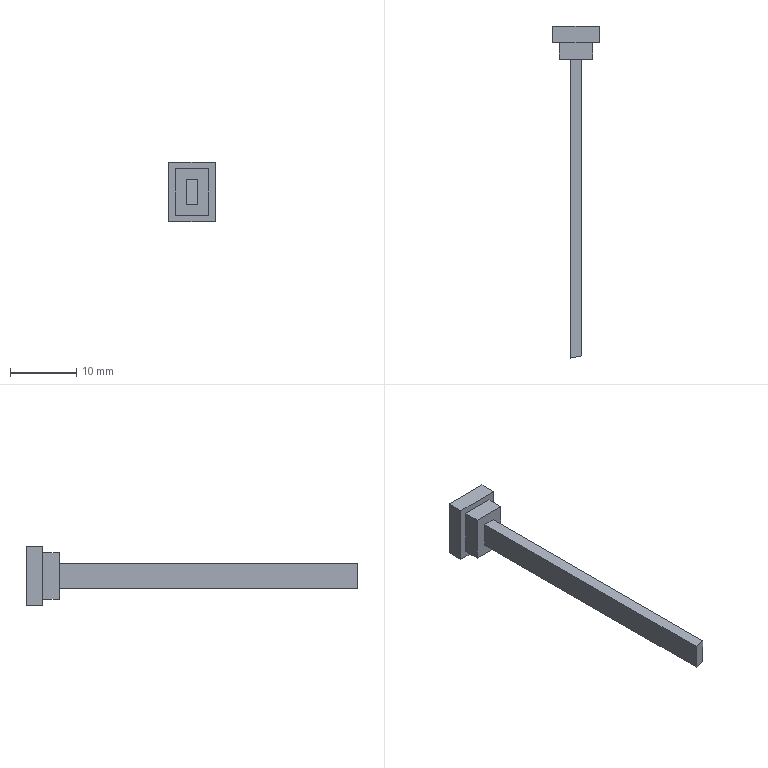Part | SolidWorks | features ICE 3, Extrusion 1 | 1 solid | 16 faces | box 7 x 50 x 9 mm | volume 546.722 mm3 | plane 16
STEP:
#1=CARTESIAN_POINT('',(-0.89,0.,-1.89));
#2=VERTEX_POINT('',#1);
#3=CARTESIAN_POINT('',(-0.89,0.,1.89));
#4=VERTEX_POINT('',#3);
#5=CARTESIAN_POINT('',(-0.89,0.,1.89));
#6=DIRECTION('',(0.,0.,1.));
#7=VECTOR('',#6,1000.);
#8=LINE('',#5,#7);
#9=EDGE_CURVE('',#2,#4,#8,.T.);
#10=ORIENTED_EDGE('',*,*,#9,.T.);
#11=CARTESIAN_POINT('',(-0.89,45.,1.89));
#12=VERTEX_POINT('',#11);
#13=CARTESIAN_POINT('',(-0.89,45.,1.89));
#14=DIRECTION('',(0.,-1.,0.));
#15=VECTOR('',#14,1000.);
#16=LINE('',#13,#15);
#17=EDGE_CURVE('',#12,#4,#16,.T.);
#18=ORIENTED_EDGE('',*,*,#17,.F.);
#19=CARTESIAN_POINT('',(-0.89,45.,-1.89));
#20=VERTEX_POINT('',#19);
#21=CARTESIAN_POINT('',(-0.89,45.,1.89));
#22=DIRECTION('',(0.,0.,1.));
#23=VECTOR('',#22,1000.);
#24=LINE('',#21,#23);
#25=EDGE_CURVE('',#20,#12,#24,.T.);
#26=ORIENTED_EDGE('',*,*,#25,.F.);
#27=CARTESIAN_POINT('',(-0.89,45.,-1.89));
#28=DIRECTION('',(0.,-1.,0.));
#29=VECTOR('',#28,1000.);
#30=LINE('',#27,#29);
#31=EDGE_CURVE('',#20,#2,#30,.T.);
#32=ORIENTED_EDGE('',*,*,#31,.T.);
#33=EDGE_LOOP('',(#10,#18,#26,#32));
#34=FACE_OUTER_BOUND('',#33,.T.);
#35=CARTESIAN_POINT('',(-0.89,45.,1.89));
#36=DIRECTION('',(1.,0.,0.));
#37=DIRECTION('',(0.,0.,-1.));
#38=AXIS2_PLACEMENT_3D('',#35,#36,#37);
#39=PLANE('',#38);
#40=ADVANCED_FACE('',(#34),#39,.F.);
#41=ORIENTED_EDGE('',*,*,#17,.T.);
#42=CARTESIAN_POINT('',(0.89,0.3139,1.89));
#43=VERTEX_POINT('',#42);
#44=CARTESIAN_POINT('',(0.89,0.3139,1.89));
#45=DIRECTION('',(-0.9848,-0.1736,0.));
#46=VECTOR('',#45,1000.);
#47=LINE('',#44,#46);
#48=EDGE_CURVE('',#43,#4,#47,.T.);
#49=ORIENTED_EDGE('',*,*,#48,.F.);
#50=CARTESIAN_POINT('',(0.89,45.,1.89));
#51=VERTEX_POINT('',#50);
#52=CARTESIAN_POINT('',(0.89,45.,1.89));
#53=DIRECTION('',(0.,-1.,0.));
#54=VECTOR('',#53,1000.);
#55=LINE('',#52,#54);
#56=EDGE_CURVE('',#51,#43,#55,.T.);
#57=ORIENTED_EDGE('',*,*,#56,.F.);
#58=CARTESIAN_POINT('',(0.89,45.,1.89));
#59=DIRECTION('',(1.,0.,0.));
#60=VECTOR('',#59,1000.);
#61=LINE('',#58,#60);
#62=EDGE_CURVE('',#12,#51,#61,.T.);
#63=ORIENTED_EDGE('',*,*,#62,.F.);
#64=EDGE_LOOP('',(#41,#49,#57,#63));
#65=FACE_OUTER_BOUND('',#64,.T.);
#66=CARTESIAN_POINT('',(0.89,45.,1.89));
#67=DIRECTION('',(0.,0.,-1.));
#68=DIRECTION('',(-1.,0.,0.));
#69=AXIS2_PLACEMENT_3D('',#66,#67,#68);
#70=PLANE('',#69);
#71=ADVANCED_FACE('',(#65),#70,.F.);
#72=ORIENTED_EDGE('',*,*,#56,.T.);
#73=CARTESIAN_POINT('',(0.89,0.3139,-1.89));
#74=VERTEX_POINT('',#73);
#75=CARTESIAN_POINT('',(0.89,0.3139,-1.89));
#76=DIRECTION('',(0.,0.,1.));
#77=VECTOR('',#76,1000.);
#78=LINE('',#75,#77);
#79=EDGE_CURVE('',#74,#43,#78,.T.);
#80=ORIENTED_EDGE('',*,*,#79,.F.);
#81=CARTESIAN_POINT('',(0.89,45.,-1.89));
#82=VERTEX_POINT('',#81);
#83=CARTESIAN_POINT('',(0.89,45.,-1.89));
#84=DIRECTION('',(0.,-1.,0.));
#85=VECTOR('',#84,1000.);
#86=LINE('',#83,#85);
#87=EDGE_CURVE('',#82,#74,#86,.T.);
#88=ORIENTED_EDGE('',*,*,#87,.F.);
#89=CARTESIAN_POINT('',(0.89,45.,-1.89));
#90=DIRECTION('',(0.,0.,-1.));
#91=VECTOR('',#90,1000.);
#92=LINE('',#89,#91);
#93=EDGE_CURVE('',#51,#82,#92,.T.);
#94=ORIENTED_EDGE('',*,*,#93,.F.);
#95=EDGE_LOOP('',(#72,#80,#88,#94));
#96=FACE_OUTER_BOUND('',#95,.T.);
#97=CARTESIAN_POINT('',(0.89,45.,-1.89));
#98=DIRECTION('',(-1.,0.,0.));
#99=DIRECTION('',(0.,0.,1.));
#100=AXIS2_PLACEMENT_3D('',#97,#98,#99);
#101=PLANE('',#100);
#102=ADVANCED_FACE('',(#96),#101,.F.);
#103=ORIENTED_EDGE('',*,*,#87,.T.);
#104=CARTESIAN_POINT('',(0.89,0.3139,-1.89));
#105=DIRECTION('',(-0.9848,-0.1736,0.));
#106=VECTOR('',#105,1000.);
#107=LINE('',#104,#106);
#108=EDGE_CURVE('',#74,#2,#107,.T.);
#109=ORIENTED_EDGE('',*,*,#108,.T.);
#110=ORIENTED_EDGE('',*,*,#31,.F.);
#111=CARTESIAN_POINT('',(-0.89,45.,-1.89));
#112=DIRECTION('',(-1.,0.,0.));
#113=VECTOR('',#112,1000.);
#114=LINE('',#111,#113);
#115=EDGE_CURVE('',#82,#20,#114,.T.);
#116=ORIENTED_EDGE('',*,*,#115,.F.);
#117=EDGE_LOOP('',(#103,#109,#110,#116));
#118=FACE_OUTER_BOUND('',#117,.T.);
#119=CARTESIAN_POINT('',(-0.89,45.,-1.89));
#120=DIRECTION('',(0.,0.,1.));
#121=DIRECTION('',(1.,0.,0.));
#122=AXIS2_PLACEMENT_3D('',#119,#120,#121);
#123=PLANE('',#122);
#124=ADVANCED_FACE('',(#118),#123,.F.);
#125=ORIENTED_EDGE('',*,*,#48,.T.);
#126=ORIENTED_EDGE('',*,*,#9,.F.);
#127=ORIENTED_EDGE('',*,*,#108,.F.);
#128=ORIENTED_EDGE('',*,*,#79,.T.);
#129=EDGE_LOOP('',(#125,#126,#127,#128));
#130=FACE_OUTER_BOUND('',#129,.T.);
#131=CARTESIAN_POINT('',(0.89,0.3139,-1.89));
#132=DIRECTION('',(-0.1736,0.9848,0.));
#133=DIRECTION('',(-0.9848,-0.1736,0.));
#134=AXIS2_PLACEMENT_3D('',#131,#132,#133);
#135=PLANE('',#134);
#136=ADVANCED_FACE('',(#130),#135,.F.);
#137=CARTESIAN_POINT('',(-2.5,45.,-3.5));
#138=VERTEX_POINT('',#137);
#139=CARTESIAN_POINT('',(-2.5,45.,3.5));
#140=VERTEX_POINT('',#139);
#141=CARTESIAN_POINT('',(-2.5,45.,-3.5));
#142=DIRECTION('',(0.,0.,1.));
#143=VECTOR('',#142,1000.);
#144=LINE('',#141,#143);
#145=EDGE_CURVE('',#138,#140,#144,.T.);
#146=ORIENTED_EDGE('',*,*,#145,.F.);
#147=CARTESIAN_POINT('',(2.5,45.,-3.5));
#148=VERTEX_POINT('',#147);
#149=CARTESIAN_POINT('',(-2.5,45.,-3.5));
#150=DIRECTION('',(-1.,0.,0.));
#151=VECTOR('',#150,1000.);
#152=LINE('',#149,#151);
#153=EDGE_CURVE('',#148,#138,#152,.T.);
#154=ORIENTED_EDGE('',*,*,#153,.F.);
#155=CARTESIAN_POINT('',(2.5,45.,3.5));
#156=VERTEX_POINT('',#155);
#157=CARTESIAN_POINT('',(2.5,45.,-3.5));
#158=DIRECTION('',(0.,0.,-1.));
#159=VECTOR('',#158,1000.);
#160=LINE('',#157,#159);
#161=EDGE_CURVE('',#156,#148,#160,.T.);
#162=ORIENTED_EDGE('',*,*,#161,.F.);
#163=CARTESIAN_POINT('',(-2.5,45.,3.5));
#164=DIRECTION('',(1.,0.,0.));
#165=VECTOR('',#164,1000.);
#166=LINE('',#163,#165);
#167=EDGE_CURVE('',#140,#156,#166,.T.);
#168=ORIENTED_EDGE('',*,*,#167,.F.);
#169=EDGE_LOOP('',(#146,#154,#162,#168));
#170=FACE_OUTER_BOUND('',#169,.T.);
#171=ORIENTED_EDGE('',*,*,#115,.T.);
#172=ORIENTED_EDGE('',*,*,#25,.T.);
#173=ORIENTED_EDGE('',*,*,#62,.T.);
#174=ORIENTED_EDGE('',*,*,#93,.T.);
#175=EDGE_LOOP('',(#171,#172,#173,#174));
#176=FACE_BOUND('',#175,.T.);
#177=CARTESIAN_POINT('',(0.,45.,0.));
#178=DIRECTION('',(0.,1.,0.));
#179=DIRECTION('',(0.,0.,1.));
#180=AXIS2_PLACEMENT_3D('',#177,#178,#179);
#181=PLANE('',#180);
#182=ADVANCED_FACE('',(#170,#176),#181,.F.);
#183=ORIENTED_EDGE('',*,*,#145,.T.);
#184=CARTESIAN_POINT('',(-2.5,47.5,3.5));
#185=VERTEX_POINT('',#184);
#186=CARTESIAN_POINT('',(-2.5,47.5,3.5));
#187=DIRECTION('',(0.,-1.,0.));
#188=VECTOR('',#187,1000.);
#189=LINE('',#186,#188);
#190=EDGE_CURVE('',#185,#140,#189,.T.);
#191=ORIENTED_EDGE('',*,*,#190,.F.);
#192=CARTESIAN_POINT('',(-2.5,47.5,-3.5));
#193=VERTEX_POINT('',#192);
#194=CARTESIAN_POINT('',(-2.5,47.5,-3.5));
#195=DIRECTION('',(0.,0.,1.));
#196=VECTOR('',#195,1000.);
#197=LINE('',#194,#196);
#198=EDGE_CURVE('',#193,#185,#197,.T.);
#199=ORIENTED_EDGE('',*,*,#198,.F.);
#200=CARTESIAN_POINT('',(-2.5,47.5,-3.5));
#201=DIRECTION('',(0.,-1.,0.));
#202=VECTOR('',#201,1000.);
#203=LINE('',#200,#202);
#204=EDGE_CURVE('',#193,#138,#203,.T.);
#205=ORIENTED_EDGE('',*,*,#204,.T.);
#206=EDGE_LOOP('',(#183,#191,#199,#205));
#207=FACE_OUTER_BOUND('',#206,.T.);
#208=CARTESIAN_POINT('',(-2.5,47.5,-3.5));
#209=DIRECTION('',(1.,0.,0.));
#210=DIRECTION('',(0.,0.,-1.));
#211=AXIS2_PLACEMENT_3D('',#208,#209,#210);
#212=PLANE('',#211);
#213=ADVANCED_FACE('',(#207),#212,.F.);
#214=ORIENTED_EDGE('',*,*,#167,.T.);
#215=CARTESIAN_POINT('',(2.5,47.5,3.5));
#216=VERTEX_POINT('',#215);
#217=CARTESIAN_POINT('',(2.5,47.5,3.5));
#218=DIRECTION('',(0.,-1.,0.));
#219=VECTOR('',#218,1000.);
#220=LINE('',#217,#219);
#221=EDGE_CURVE('',#216,#156,#220,.T.);
#222=ORIENTED_EDGE('',*,*,#221,.F.);
#223=CARTESIAN_POINT('',(-2.5,47.5,3.5));
#224=DIRECTION('',(1.,0.,0.));
#225=VECTOR('',#224,1000.);
#226=LINE('',#223,#225);
#227=EDGE_CURVE('',#185,#216,#226,.T.);
#228=ORIENTED_EDGE('',*,*,#227,.F.);
#229=ORIENTED_EDGE('',*,*,#190,.T.);
#230=EDGE_LOOP('',(#214,#222,#228,#229));
#231=FACE_OUTER_BOUND('',#230,.T.);
#232=CARTESIAN_POINT('',(-2.5,47.5,3.5));
#233=DIRECTION('',(0.,0.,-1.));
#234=DIRECTION('',(-1.,0.,0.));
#235=AXIS2_PLACEMENT_3D('',#232,#233,#234);
#236=PLANE('',#235);
#237=ADVANCED_FACE('',(#231),#236,.F.);
#238=ORIENTED_EDGE('',*,*,#161,.T.);
#239=CARTESIAN_POINT('',(2.5,47.5,-3.5));
#240=VERTEX_POINT('',#239);
#241=CARTESIAN_POINT('',(2.5,47.5,-3.5));
#242=DIRECTION('',(0.,-1.,0.));
#243=VECTOR('',#242,1000.);
#244=LINE('',#241,#243);
#245=EDGE_CURVE('',#240,#148,#244,.T.);
#246=ORIENTED_EDGE('',*,*,#245,.F.);
#247=CARTESIAN_POINT('',(2.5,47.5,-3.5));
#248=DIRECTION('',(0.,0.,-1.));
#249=VECTOR('',#248,1000.);
#250=LINE('',#247,#249);
#251=EDGE_CURVE('',#216,#240,#250,.T.);
#252=ORIENTED_EDGE('',*,*,#251,.F.);
#253=ORIENTED_EDGE('',*,*,#221,.T.);
#254=EDGE_LOOP('',(#238,#246,#252,#253));
#255=FACE_OUTER_BOUND('',#254,.T.);
#256=CARTESIAN_POINT('',(2.5,47.5,-3.5));
#257=DIRECTION('',(-1.,0.,0.));
#258=DIRECTION('',(0.,0.,1.));
#259=AXIS2_PLACEMENT_3D('',#256,#257,#258);
#260=PLANE('',#259);
#261=ADVANCED_FACE('',(#255),#260,.F.);
#262=ORIENTED_EDGE('',*,*,#153,.T.);
#263=ORIENTED_EDGE('',*,*,#204,.F.);
#264=CARTESIAN_POINT('',(-2.5,47.5,-3.5));
#265=DIRECTION('',(-1.,0.,0.));
#266=VECTOR('',#265,1000.);
#267=LINE('',#264,#266);
#268=EDGE_CURVE('',#240,#193,#267,.T.);
#269=ORIENTED_EDGE('',*,*,#268,.F.);
#270=ORIENTED_EDGE('',*,*,#245,.T.);
#271=EDGE_LOOP('',(#262,#263,#269,#270));
#272=FACE_OUTER_BOUND('',#271,.T.);
#273=CARTESIAN_POINT('',(-2.5,47.5,-3.5));
#274=DIRECTION('',(0.,0.,1.));
#275=DIRECTION('',(1.,0.,0.));
#276=AXIS2_PLACEMENT_3D('',#273,#274,#275);
#277=PLANE('',#276);
#278=ADVANCED_FACE('',(#272),#277,.F.);
#279=CARTESIAN_POINT('',(-3.5,47.5,-4.5));
#280=VERTEX_POINT('',#279);
#281=CARTESIAN_POINT('',(-3.5,47.5,4.5));
#282=VERTEX_POINT('',#281);
#283=CARTESIAN_POINT('',(-3.5,47.5,-4.5));
#284=DIRECTION('',(0.,0.,1.));
#285=VECTOR('',#284,1000.);
#286=LINE('',#283,#285);
#287=EDGE_CURVE('',#280,#282,#286,.T.);
#288=ORIENTED_EDGE('',*,*,#287,.F.);
#289=CARTESIAN_POINT('',(3.5,47.5,-4.5));
#290=VERTEX_POINT('',#289);
#291=CARTESIAN_POINT('',(-3.5,47.5,-4.5));
#292=DIRECTION('',(-1.,0.,0.));
#293=VECTOR('',#292,1000.);
#294=LINE('',#291,#293);
#295=EDGE_CURVE('',#290,#280,#294,.T.);
#296=ORIENTED_EDGE('',*,*,#295,.F.);
#297=CARTESIAN_POINT('',(3.5,47.5,4.5));
#298=VERTEX_POINT('',#297);
#299=CARTESIAN_POINT('',(3.5,47.5,-4.5));
#300=DIRECTION('',(0.,0.,-1.));
#301=VECTOR('',#300,1000.);
#302=LINE('',#299,#301);
#303=EDGE_CURVE('',#298,#290,#302,.T.);
#304=ORIENTED_EDGE('',*,*,#303,.F.);
#305=CARTESIAN_POINT('',(-3.5,47.5,4.5));
#306=DIRECTION('',(1.,0.,0.));
#307=VECTOR('',#306,1000.);
#308=LINE('',#305,#307);
#309=EDGE_CURVE('',#282,#298,#308,.T.);
#310=ORIENTED_EDGE('',*,*,#309,.F.);
#311=EDGE_LOOP('',(#288,#296,#304,#310));
#312=FACE_OUTER_BOUND('',#311,.T.);
#313=ORIENTED_EDGE('',*,*,#268,.T.);
#314=ORIENTED_EDGE('',*,*,#198,.T.);
#315=ORIENTED_EDGE('',*,*,#227,.T.);
#316=ORIENTED_EDGE('',*,*,#251,.T.);
#317=EDGE_LOOP('',(#313,#314,#315,#316));
#318=FACE_BOUND('',#317,.T.);
#319=CARTESIAN_POINT('',(0.,47.5,0.));
#320=DIRECTION('',(0.,1.,0.));
#321=DIRECTION('',(0.,0.,1.));
#322=AXIS2_PLACEMENT_3D('',#319,#320,#321);
#323=PLANE('',#322);
#324=ADVANCED_FACE('',(#312,#318),#323,.F.);
#325=ORIENTED_EDGE('',*,*,#287,.T.);
#326=CARTESIAN_POINT('',(-3.5,50.,4.5));
#327=VERTEX_POINT('',#326);
#328=CARTESIAN_POINT('',(-3.5,50.,4.5));
#329=DIRECTION('',(0.,-1.,0.));
#330=VECTOR('',#329,1000.);
#331=LINE('',#328,#330);
#332=EDGE_CURVE('',#327,#282,#331,.T.);
#333=ORIENTED_EDGE('',*,*,#332,.F.);
#334=CARTESIAN_POINT('',(-3.5,50.,-4.5));
#335=VERTEX_POINT('',#334);
#336=CARTESIAN_POINT('',(-3.5,50.,-4.5));
#337=DIRECTION('',(0.,0.,1.));
#338=VECTOR('',#337,1000.);
#339=LINE('',#336,#338);
#340=EDGE_CURVE('',#335,#327,#339,.T.);
#341=ORIENTED_EDGE('',*,*,#340,.F.);
#342=CARTESIAN_POINT('',(-3.5,50.,-4.5));
#343=DIRECTION('',(0.,-1.,0.));
#344=VECTOR('',#343,1000.);
#345=LINE('',#342,#344);
#346=EDGE_CURVE('',#335,#280,#345,.T.);
#347=ORIENTED_EDGE('',*,*,#346,.T.);
#348=EDGE_LOOP('',(#325,#333,#341,#347));
#349=FACE_OUTER_BOUND('',#348,.T.);
#350=CARTESIAN_POINT('',(-3.5,50.,-4.5));
#351=DIRECTION('',(1.,0.,0.));
#352=DIRECTION('',(0.,0.,-1.));
#353=AXIS2_PLACEMENT_3D('',#350,#351,#352);
#354=PLANE('',#353);
#355=ADVANCED_FACE('',(#349),#354,.F.);
#356=ORIENTED_EDGE('',*,*,#309,.T.);
#357=CARTESIAN_POINT('',(3.5,50.,4.5));
#358=VERTEX_POINT('',#357);
#359=CARTESIAN_POINT('',(3.5,50.,4.5));
#360=DIRECTION('',(0.,-1.,0.));
#361=VECTOR('',#360,1000.);
#362=LINE('',#359,#361);
#363=EDGE_CURVE('',#358,#298,#362,.T.);
#364=ORIENTED_EDGE('',*,*,#363,.F.);
#365=CARTESIAN_POINT('',(-3.5,50.,4.5));
#366=DIRECTION('',(1.,0.,0.));
#367=VECTOR('',#366,1000.);
#368=LINE('',#365,#367);
#369=EDGE_CURVE('',#327,#358,#368,.T.);
#370=ORIENTED_EDGE('',*,*,#369,.F.);
#371=ORIENTED_EDGE('',*,*,#332,.T.);
#372=EDGE_LOOP('',(#356,#364,#370,#371));
#373=FACE_OUTER_BOUND('',#372,.T.);
#374=CARTESIAN_POINT('',(-3.5,50.,4.5));
#375=DIRECTION('',(0.,0.,-1.));
#376=DIRECTION('',(-1.,0.,0.));
#377=AXIS2_PLACEMENT_3D('',#374,#375,#376);
#378=PLANE('',#377);
#379=ADVANCED_FACE('',(#373),#378,.F.);
#380=ORIENTED_EDGE('',*,*,#303,.T.);
#381=CARTESIAN_POINT('',(3.5,50.,-4.5));
#382=VERTEX_POINT('',#381);
#383=CARTESIAN_POINT('',(3.5,50.,-4.5));
#384=DIRECTION('',(0.,-1.,0.));
#385=VECTOR('',#384,1000.);
#386=LINE('',#383,#385);
#387=EDGE_CURVE('',#382,#290,#386,.T.);
#388=ORIENTED_EDGE('',*,*,#387,.F.);
#389=CARTESIAN_POINT('',(3.5,50.,-4.5));
#390=DIRECTION('',(0.,0.,-1.));
#391=VECTOR('',#390,1000.);
#392=LINE('',#389,#391);
#393=EDGE_CURVE('',#358,#382,#392,.T.);
#394=ORIENTED_EDGE('',*,*,#393,.F.);
#395=ORIENTED_EDGE('',*,*,#363,.T.);
#396=EDGE_LOOP('',(#380,#388,#394,#395));
#397=FACE_OUTER_BOUND('',#396,.T.);
#398=CARTESIAN_POINT('',(3.5,50.,-4.5));
#399=DIRECTION('',(-1.,0.,0.));
#400=DIRECTION('',(0.,0.,1.));
#401=AXIS2_PLACEMENT_3D('',#398,#399,#400);
#402=PLANE('',#401);
#403=ADVANCED_FACE('',(#397),#402,.F.);
#404=ORIENTED_EDGE('',*,*,#295,.T.);
#405=ORIENTED_EDGE('',*,*,#346,.F.);
#406=CARTESIAN_POINT('',(-3.5,50.,-4.5));
#407=DIRECTION('',(-1.,0.,0.));
#408=VECTOR('',#407,1000.);
#409=LINE('',#406,#408);
#410=EDGE_CURVE('',#382,#335,#409,.T.);
#411=ORIENTED_EDGE('',*,*,#410,.F.);
#412=ORIENTED_EDGE('',*,*,#387,.T.);
#413=EDGE_LOOP('',(#404,#405,#411,#412));
#414=FACE_OUTER_BOUND('',#413,.T.);
#415=CARTESIAN_POINT('',(-3.5,50.,-4.5));
#416=DIRECTION('',(0.,0.,1.));
#417=DIRECTION('',(1.,0.,0.));
#418=AXIS2_PLACEMENT_3D('',#415,#416,#417);
#419=PLANE('',#418);
#420=ADVANCED_FACE('',(#414),#419,.F.);
#421=ORIENTED_EDGE('',*,*,#340,.T.);
#422=ORIENTED_EDGE('',*,*,#369,.T.);
#423=ORIENTED_EDGE('',*,*,#393,.T.);
#424=ORIENTED_EDGE('',*,*,#410,.T.);
#425=EDGE_LOOP('',(#421,#422,#423,#424));
#426=FACE_OUTER_BOUND('',#425,.T.);
#427=CARTESIAN_POINT('',(0.,50.,0.));
#428=DIRECTION('',(0.,1.,0.));
#429=DIRECTION('',(0.,0.,1.));
#430=AXIS2_PLACEMENT_3D('',#427,#428,#429);
#431=PLANE('',#430);
#432=ADVANCED_FACE('',(#426),#431,.T.);
#433=CLOSED_SHELL('',(#40,#71,#102,#124,#136,#182,#213,#237,#261,#278,#324,#355,#379,#403,#420,#432));
#434=MANIFOLD_SOLID_BREP('',#433);
#435=CARTESIAN_POINT('',(0.,0.,0.));
#436=DIRECTION('',(0.,0.,1.));
#437=DIRECTION('',(1.,0.,0.));
#438=AXIS2_PLACEMENT_3D('',#435,#436,#437);
#439=(LENGTH_UNIT()NAMED_UNIT(*)SI_UNIT(.MILLI.,.METRE.));
#440=UNCERTAINTY_MEASURE_WITH_UNIT(LENGTH_MEASURE(0.00001),#439,'','');
#441=(NAMED_UNIT(*)PLANE_ANGLE_UNIT()SI_UNIT($,.RADIAN.));
#442=(NAMED_UNIT(*)SI_UNIT($,.STERADIAN.)SOLID_ANGLE_UNIT());
#443=(GEOMETRIC_REPRESENTATION_CONTEXT(3)GLOBAL_UNCERTAINTY_ASSIGNED_CONTEXT((#440))GLOBAL_UNIT_ASSIGNED_CONTEXT((#439,#441,#442))REPRESENTATION_CONTEXT('',''));
#444=ADVANCED_BREP_SHAPE_REPRESENTATION('',(#434,#438),#443);